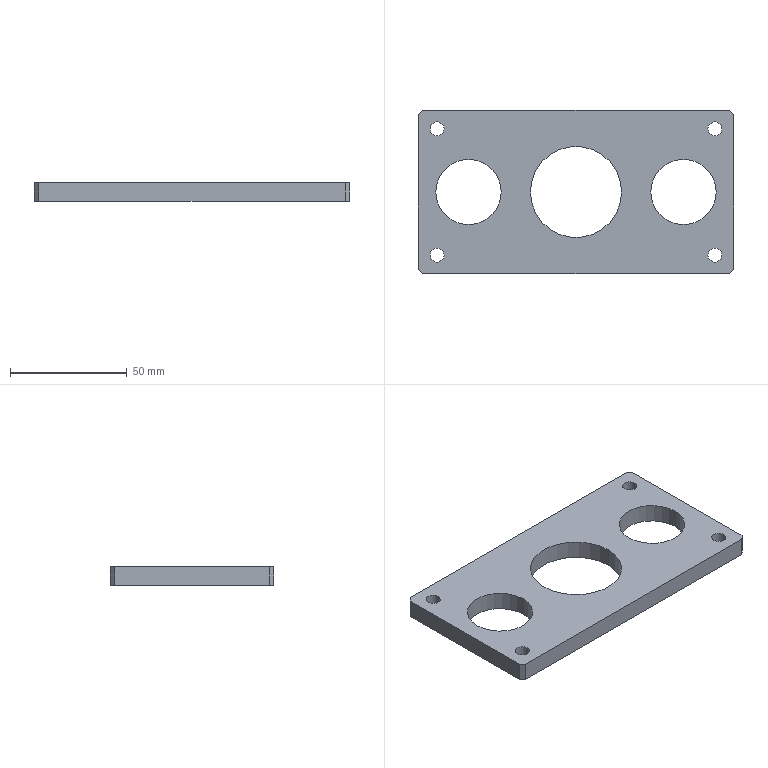Part | SolidWorks | features ICE 3, Chamfer 1, Extrusion 1 | 1 solid | 24 faces | box 135 x 70 x 8 mm | volume 55222 mm3 | cylinder 14 | plane 10 | commonest cylinder face diameters 6 x8 28 x4 39 x2
STEP:
#1=CARTESIAN_POINT('',(56.5,27.,0.));
#2=VERTEX_POINT('',#1);
#3=CARTESIAN_POINT('',(62.5,27.,0.));
#4=VERTEX_POINT('',#3);
#5=CARTESIAN_POINT('',(59.5,27.,0.));
#6=DIRECTION('',(0.,0.,1.));
#7=DIRECTION('',(-1.,0.,0.));
#8=AXIS2_PLACEMENT_3D('',#5,#6,#7);
#9=CIRCLE('',#8,3.);
#10=EDGE_CURVE('',#2,#4,#9,.T.);
#11=ORIENTED_EDGE('',*,*,#10,.F.);
#12=CARTESIAN_POINT('',(56.5,27.,8.));
#13=VERTEX_POINT('',#12);
#14=CARTESIAN_POINT('',(56.5,27.,-0.001));
#15=DIRECTION('',(0.,0.,1.));
#16=VECTOR('',#15,1000.);
#17=LINE('',#14,#16);
#18=EDGE_CURVE('',#2,#13,#17,.T.);
#19=ORIENTED_EDGE('',*,*,#18,.T.);
#20=CARTESIAN_POINT('',(62.5,27.,8.));
#21=VERTEX_POINT('',#20);
#22=CARTESIAN_POINT('',(59.5,27.,8.));
#23=DIRECTION('',(0.,0.,1.));
#24=DIRECTION('',(-1.,0.,0.));
#25=AXIS2_PLACEMENT_3D('',#22,#23,#24);
#26=CIRCLE('',#25,3.);
#27=EDGE_CURVE('',#13,#21,#26,.T.);
#28=ORIENTED_EDGE('',*,*,#27,.T.);
#29=CARTESIAN_POINT('',(62.5,27.,-0.001));
#30=DIRECTION('',(0.,0.,1.));
#31=VECTOR('',#30,1000.);
#32=LINE('',#29,#31);
#33=EDGE_CURVE('',#4,#21,#32,.T.);
#34=ORIENTED_EDGE('',*,*,#33,.F.);
#35=EDGE_LOOP('',(#11,#19,#28,#34));
#36=FACE_OUTER_BOUND('',#35,.T.);
#37=CARTESIAN_POINT('',(59.5,27.,-0.001));
#38=DIRECTION('',(0.,0.,1.));
#39=DIRECTION('',(1.,0.,0.));
#40=AXIS2_PLACEMENT_3D('',#37,#38,#39);
#41=CYLINDRICAL_SURFACE('',#40,3.);
#42=ADVANCED_FACE('',(#36),#41,.F.);
#43=CARTESIAN_POINT('',(56.5,-27.,0.));
#44=VERTEX_POINT('',#43);
#45=CARTESIAN_POINT('',(62.5,-27.,0.));
#46=VERTEX_POINT('',#45);
#47=CARTESIAN_POINT('',(59.5,-27.,0.));
#48=DIRECTION('',(0.,0.,1.));
#49=DIRECTION('',(-1.,0.,0.));
#50=AXIS2_PLACEMENT_3D('',#47,#48,#49);
#51=CIRCLE('',#50,3.);
#52=EDGE_CURVE('',#44,#46,#51,.T.);
#53=ORIENTED_EDGE('',*,*,#52,.F.);
#54=CARTESIAN_POINT('',(56.5,-27.,8.));
#55=VERTEX_POINT('',#54);
#56=CARTESIAN_POINT('',(56.5,-27.,-0.001));
#57=DIRECTION('',(0.,0.,1.));
#58=VECTOR('',#57,1000.);
#59=LINE('',#56,#58);
#60=EDGE_CURVE('',#44,#55,#59,.T.);
#61=ORIENTED_EDGE('',*,*,#60,.T.);
#62=CARTESIAN_POINT('',(62.5,-27.,8.));
#63=VERTEX_POINT('',#62);
#64=CARTESIAN_POINT('',(59.5,-27.,8.));
#65=DIRECTION('',(0.,0.,1.));
#66=DIRECTION('',(-1.,0.,0.));
#67=AXIS2_PLACEMENT_3D('',#64,#65,#66);
#68=CIRCLE('',#67,3.);
#69=EDGE_CURVE('',#55,#63,#68,.T.);
#70=ORIENTED_EDGE('',*,*,#69,.T.);
#71=CARTESIAN_POINT('',(62.5,-27.,-0.001));
#72=DIRECTION('',(0.,0.,1.));
#73=VECTOR('',#72,1000.);
#74=LINE('',#71,#73);
#75=EDGE_CURVE('',#46,#63,#74,.T.);
#76=ORIENTED_EDGE('',*,*,#75,.F.);
#77=EDGE_LOOP('',(#53,#61,#70,#76));
#78=FACE_OUTER_BOUND('',#77,.T.);
#79=CARTESIAN_POINT('',(59.5,-27.,-0.001));
#80=DIRECTION('',(0.,0.,1.));
#81=DIRECTION('',(1.,0.,0.));
#82=AXIS2_PLACEMENT_3D('',#79,#80,#81);
#83=CYLINDRICAL_SURFACE('',#82,3.);
#84=ADVANCED_FACE('',(#78),#83,.F.);
#85=CARTESIAN_POINT('',(-62.5,-27.,0.));
#86=VERTEX_POINT('',#85);
#87=CARTESIAN_POINT('',(-56.5,-27.,0.));
#88=VERTEX_POINT('',#87);
#89=CARTESIAN_POINT('',(-59.5,-27.,0.));
#90=DIRECTION('',(0.,0.,1.));
#91=DIRECTION('',(-1.,0.,0.));
#92=AXIS2_PLACEMENT_3D('',#89,#90,#91);
#93=CIRCLE('',#92,3.);
#94=EDGE_CURVE('',#86,#88,#93,.T.);
#95=ORIENTED_EDGE('',*,*,#94,.F.);
#96=CARTESIAN_POINT('',(-62.5,-27.,8.));
#97=VERTEX_POINT('',#96);
#98=CARTESIAN_POINT('',(-62.5,-27.,-0.001));
#99=DIRECTION('',(0.,0.,1.));
#100=VECTOR('',#99,1000.);
#101=LINE('',#98,#100);
#102=EDGE_CURVE('',#86,#97,#101,.T.);
#103=ORIENTED_EDGE('',*,*,#102,.T.);
#104=CARTESIAN_POINT('',(-56.5,-27.,8.));
#105=VERTEX_POINT('',#104);
#106=CARTESIAN_POINT('',(-59.5,-27.,8.));
#107=DIRECTION('',(0.,0.,1.));
#108=DIRECTION('',(1.,0.,0.));
#109=AXIS2_PLACEMENT_3D('',#106,#107,#108);
#110=CIRCLE('',#109,3.);
#111=EDGE_CURVE('',#97,#105,#110,.T.);
#112=ORIENTED_EDGE('',*,*,#111,.T.);
#113=CARTESIAN_POINT('',(-56.5,-27.,-0.001));
#114=DIRECTION('',(0.,0.,1.));
#115=VECTOR('',#114,1000.);
#116=LINE('',#113,#115);
#117=EDGE_CURVE('',#88,#105,#116,.T.);
#118=ORIENTED_EDGE('',*,*,#117,.F.);
#119=EDGE_LOOP('',(#95,#103,#112,#118));
#120=FACE_OUTER_BOUND('',#119,.T.);
#121=CARTESIAN_POINT('',(-59.5,-27.,-0.001));
#122=DIRECTION('',(0.,0.,1.));
#123=DIRECTION('',(1.,0.,0.));
#124=AXIS2_PLACEMENT_3D('',#121,#122,#123);
#125=CYLINDRICAL_SURFACE('',#124,3.);
#126=ADVANCED_FACE('',(#120),#125,.F.);
#127=CARTESIAN_POINT('',(-62.5,27.,0.));
#128=VERTEX_POINT('',#127);
#129=CARTESIAN_POINT('',(-56.5,27.,0.));
#130=VERTEX_POINT('',#129);
#131=CARTESIAN_POINT('',(-59.5,27.,0.));
#132=DIRECTION('',(0.,0.,1.));
#133=DIRECTION('',(-1.,0.,0.));
#134=AXIS2_PLACEMENT_3D('',#131,#132,#133);
#135=CIRCLE('',#134,3.);
#136=EDGE_CURVE('',#128,#130,#135,.T.);
#137=ORIENTED_EDGE('',*,*,#136,.F.);
#138=CARTESIAN_POINT('',(-62.5,27.,8.));
#139=VERTEX_POINT('',#138);
#140=CARTESIAN_POINT('',(-62.5,27.,-0.001));
#141=DIRECTION('',(0.,0.,1.));
#142=VECTOR('',#141,1000.);
#143=LINE('',#140,#142);
#144=EDGE_CURVE('',#128,#139,#143,.T.);
#145=ORIENTED_EDGE('',*,*,#144,.T.);
#146=CARTESIAN_POINT('',(-56.5,27.,8.));
#147=VERTEX_POINT('',#146);
#148=CARTESIAN_POINT('',(-59.5,27.,8.));
#149=DIRECTION('',(0.,0.,1.));
#150=DIRECTION('',(1.,0.,0.));
#151=AXIS2_PLACEMENT_3D('',#148,#149,#150);
#152=CIRCLE('',#151,3.);
#153=EDGE_CURVE('',#139,#147,#152,.T.);
#154=ORIENTED_EDGE('',*,*,#153,.T.);
#155=CARTESIAN_POINT('',(-56.5,27.,-0.001));
#156=DIRECTION('',(0.,0.,1.));
#157=VECTOR('',#156,1000.);
#158=LINE('',#155,#157);
#159=EDGE_CURVE('',#130,#147,#158,.T.);
#160=ORIENTED_EDGE('',*,*,#159,.F.);
#161=EDGE_LOOP('',(#137,#145,#154,#160));
#162=FACE_OUTER_BOUND('',#161,.T.);
#163=CARTESIAN_POINT('',(-59.5,27.,-0.001));
#164=DIRECTION('',(0.,0.,1.));
#165=DIRECTION('',(1.,0.,0.));
#166=AXIS2_PLACEMENT_3D('',#163,#164,#165);
#167=CYLINDRICAL_SURFACE('',#166,3.);
#168=ADVANCED_FACE('',(#162),#167,.F.);
#169=CARTESIAN_POINT('',(32.,0.,0.));
#170=VERTEX_POINT('',#169);
#171=CARTESIAN_POINT('',(60.,0.,0.));
#172=VERTEX_POINT('',#171);
#173=CARTESIAN_POINT('',(46.,0.,0.));
#174=DIRECTION('',(0.,0.,1.));
#175=DIRECTION('',(-1.,0.,0.));
#176=AXIS2_PLACEMENT_3D('',#173,#174,#175);
#177=CIRCLE('',#176,14.);
#178=EDGE_CURVE('',#170,#172,#177,.T.);
#179=ORIENTED_EDGE('',*,*,#178,.F.);
#180=CARTESIAN_POINT('',(32.,0.,8.));
#181=VERTEX_POINT('',#180);
#182=CARTESIAN_POINT('',(32.,0.,-0.001));
#183=DIRECTION('',(0.,0.,1.));
#184=VECTOR('',#183,1000.);
#185=LINE('',#182,#184);
#186=EDGE_CURVE('',#170,#181,#185,.T.);
#187=ORIENTED_EDGE('',*,*,#186,.T.);
#188=CARTESIAN_POINT('',(60.,0.,8.));
#189=VERTEX_POINT('',#188);
#190=CARTESIAN_POINT('',(46.,0.,8.));
#191=DIRECTION('',(0.,0.,1.));
#192=DIRECTION('',(1.,0.,0.));
#193=AXIS2_PLACEMENT_3D('',#190,#191,#192);
#194=CIRCLE('',#193,14.);
#195=EDGE_CURVE('',#181,#189,#194,.T.);
#196=ORIENTED_EDGE('',*,*,#195,.T.);
#197=CARTESIAN_POINT('',(60.,0.,-0.001));
#198=DIRECTION('',(0.,0.,1.));
#199=VECTOR('',#198,1000.);
#200=LINE('',#197,#199);
#201=EDGE_CURVE('',#172,#189,#200,.T.);
#202=ORIENTED_EDGE('',*,*,#201,.F.);
#203=EDGE_LOOP('',(#179,#187,#196,#202));
#204=FACE_OUTER_BOUND('',#203,.T.);
#205=CARTESIAN_POINT('',(46.,0.,-0.001));
#206=DIRECTION('',(0.,0.,1.));
#207=DIRECTION('',(1.,0.,0.));
#208=AXIS2_PLACEMENT_3D('',#205,#206,#207);
#209=CYLINDRICAL_SURFACE('',#208,14.);
#210=ADVANCED_FACE('',(#204),#209,.F.);
#211=CARTESIAN_POINT('',(-60.,0.,0.));
#212=VERTEX_POINT('',#211);
#213=CARTESIAN_POINT('',(-32.,0.,0.));
#214=VERTEX_POINT('',#213);
#215=CARTESIAN_POINT('',(-46.,0.,0.));
#216=DIRECTION('',(0.,0.,1.));
#217=DIRECTION('',(-1.,0.,0.));
#218=AXIS2_PLACEMENT_3D('',#215,#216,#217);
#219=CIRCLE('',#218,14.);
#220=EDGE_CURVE('',#212,#214,#219,.T.);
#221=ORIENTED_EDGE('',*,*,#220,.F.);
#222=CARTESIAN_POINT('',(-60.,0.,8.));
#223=VERTEX_POINT('',#222);
#224=CARTESIAN_POINT('',(-60.,0.,-0.001));
#225=DIRECTION('',(0.,0.,1.));
#226=VECTOR('',#225,1000.);
#227=LINE('',#224,#226);
#228=EDGE_CURVE('',#212,#223,#227,.T.);
#229=ORIENTED_EDGE('',*,*,#228,.T.);
#230=CARTESIAN_POINT('',(-32.,0.,8.));
#231=VERTEX_POINT('',#230);
#232=CARTESIAN_POINT('',(-46.,0.,8.));
#233=DIRECTION('',(0.,0.,1.));
#234=DIRECTION('',(1.,0.,0.));
#235=AXIS2_PLACEMENT_3D('',#232,#233,#234);
#236=CIRCLE('',#235,14.);
#237=EDGE_CURVE('',#223,#231,#236,.T.);
#238=ORIENTED_EDGE('',*,*,#237,.T.);
#239=CARTESIAN_POINT('',(-32.,0.,-0.001));
#240=DIRECTION('',(0.,0.,1.));
#241=VECTOR('',#240,1000.);
#242=LINE('',#239,#241);
#243=EDGE_CURVE('',#214,#231,#242,.T.);
#244=ORIENTED_EDGE('',*,*,#243,.F.);
#245=EDGE_LOOP('',(#221,#229,#238,#244));
#246=FACE_OUTER_BOUND('',#245,.T.);
#247=CARTESIAN_POINT('',(-46.,0.,-0.001));
#248=DIRECTION('',(0.,0.,1.));
#249=DIRECTION('',(1.,0.,0.));
#250=AXIS2_PLACEMENT_3D('',#247,#248,#249);
#251=CYLINDRICAL_SURFACE('',#250,14.);
#252=ADVANCED_FACE('',(#246),#251,.F.);
#253=CARTESIAN_POINT('',(-19.5,0.,0.));
#254=VERTEX_POINT('',#253);
#255=CARTESIAN_POINT('',(19.5,0.,0.));
#256=VERTEX_POINT('',#255);
#257=CARTESIAN_POINT('',(0.,0.,0.));
#258=DIRECTION('',(0.,0.,1.));
#259=DIRECTION('',(-1.,0.,0.));
#260=AXIS2_PLACEMENT_3D('',#257,#258,#259);
#261=CIRCLE('',#260,19.5);
#262=EDGE_CURVE('',#254,#256,#261,.T.);
#263=ORIENTED_EDGE('',*,*,#262,.F.);
#264=CARTESIAN_POINT('',(-19.5,0.,8.));
#265=VERTEX_POINT('',#264);
#266=CARTESIAN_POINT('',(-19.5,0.,-0.001));
#267=DIRECTION('',(0.,0.,1.));
#268=VECTOR('',#267,1000.);
#269=LINE('',#266,#268);
#270=EDGE_CURVE('',#254,#265,#269,.T.);
#271=ORIENTED_EDGE('',*,*,#270,.T.);
#272=CARTESIAN_POINT('',(19.5,0.,8.));
#273=VERTEX_POINT('',#272);
#274=CARTESIAN_POINT('',(0.,0.,8.));
#275=DIRECTION('',(0.,0.,1.));
#276=DIRECTION('',(1.,0.,0.));
#277=AXIS2_PLACEMENT_3D('',#274,#275,#276);
#278=CIRCLE('',#277,19.5);
#279=EDGE_CURVE('',#265,#273,#278,.T.);
#280=ORIENTED_EDGE('',*,*,#279,.T.);
#281=CARTESIAN_POINT('',(19.5,0.,-0.001));
#282=DIRECTION('',(0.,0.,1.));
#283=VECTOR('',#282,1000.);
#284=LINE('',#281,#283);
#285=EDGE_CURVE('',#256,#273,#284,.T.);
#286=ORIENTED_EDGE('',*,*,#285,.F.);
#287=EDGE_LOOP('',(#263,#271,#280,#286));
#288=FACE_OUTER_BOUND('',#287,.T.);
#289=CARTESIAN_POINT('',(0.,0.,-0.001));
#290=DIRECTION('',(0.,0.,1.));
#291=DIRECTION('',(1.,0.,0.));
#292=AXIS2_PLACEMENT_3D('',#289,#290,#291);
#293=CYLINDRICAL_SURFACE('',#292,19.5);
#294=ADVANCED_FACE('',(#288),#293,.F.);
#295=CARTESIAN_POINT('',(67.5,-33.,8.));
#296=VERTEX_POINT('',#295);
#297=CARTESIAN_POINT('',(67.5,33.,8.));
#298=VERTEX_POINT('',#297);
#299=CARTESIAN_POINT('',(67.5,-35.,8.));
#300=DIRECTION('',(0.,1.,0.));
#301=VECTOR('',#300,1000.);
#302=LINE('',#299,#301);
#303=EDGE_CURVE('',#296,#298,#302,.T.);
#304=ORIENTED_EDGE('',*,*,#303,.F.);
#305=CARTESIAN_POINT('',(67.5,-33.,0.));
#306=VERTEX_POINT('',#305);
#307=CARTESIAN_POINT('',(67.5,-33.,8.));
#308=DIRECTION('',(0.,0.,-1.));
#309=VECTOR('',#308,1000.);
#310=LINE('',#307,#309);
#311=EDGE_CURVE('',#296,#306,#310,.T.);
#312=ORIENTED_EDGE('',*,*,#311,.T.);
#313=CARTESIAN_POINT('',(67.5,33.,0.));
#314=VERTEX_POINT('',#313);
#315=CARTESIAN_POINT('',(67.5,-35.,0.));
#316=DIRECTION('',(0.,1.,0.));
#317=VECTOR('',#316,1000.);
#318=LINE('',#315,#317);
#319=EDGE_CURVE('',#306,#314,#318,.T.);
#320=ORIENTED_EDGE('',*,*,#319,.T.);
#321=CARTESIAN_POINT('',(67.5,33.,8.));
#322=DIRECTION('',(0.,0.,1.));
#323=VECTOR('',#322,1000.);
#324=LINE('',#321,#323);
#325=EDGE_CURVE('',#314,#298,#324,.T.);
#326=ORIENTED_EDGE('',*,*,#325,.T.);
#327=EDGE_LOOP('',(#304,#312,#320,#326));
#328=FACE_OUTER_BOUND('',#327,.T.);
#329=CARTESIAN_POINT('',(67.5,-35.,8.));
#330=DIRECTION('',(-1.,0.,0.));
#331=DIRECTION('',(0.,0.,1.));
#332=AXIS2_PLACEMENT_3D('',#329,#330,#331);
#333=PLANE('',#332);
#334=ADVANCED_FACE('',(#328),#333,.F.);
#335=CARTESIAN_POINT('',(65.5,35.,8.));
#336=VERTEX_POINT('',#335);
#337=CARTESIAN_POINT('',(-65.5,35.,8.));
#338=VERTEX_POINT('',#337);
#339=CARTESIAN_POINT('',(-67.5,35.,8.));
#340=DIRECTION('',(-1.,0.,0.));
#341=VECTOR('',#340,1000.);
#342=LINE('',#339,#341);
#343=EDGE_CURVE('',#336,#338,#342,.T.);
#344=ORIENTED_EDGE('',*,*,#343,.F.);
#345=CARTESIAN_POINT('',(65.5,35.,0.));
#346=VERTEX_POINT('',#345);
#347=CARTESIAN_POINT('',(65.5,35.,8.));
#348=DIRECTION('',(0.,0.,-1.));
#349=VECTOR('',#348,1000.);
#350=LINE('',#347,#349);
#351=EDGE_CURVE('',#336,#346,#350,.T.);
#352=ORIENTED_EDGE('',*,*,#351,.T.);
#353=CARTESIAN_POINT('',(-65.5,35.,0.));
#354=VERTEX_POINT('',#353);
#355=CARTESIAN_POINT('',(-67.5,35.,0.));
#356=DIRECTION('',(-1.,0.,0.));
#357=VECTOR('',#356,1000.);
#358=LINE('',#355,#357);
#359=EDGE_CURVE('',#346,#354,#358,.T.);
#360=ORIENTED_EDGE('',*,*,#359,.T.);
#361=CARTESIAN_POINT('',(-65.5,35.,8.));
#362=DIRECTION('',(0.,0.,1.));
#363=VECTOR('',#362,1000.);
#364=LINE('',#361,#363);
#365=EDGE_CURVE('',#354,#338,#364,.T.);
#366=ORIENTED_EDGE('',*,*,#365,.T.);
#367=EDGE_LOOP('',(#344,#352,#360,#366));
#368=FACE_OUTER_BOUND('',#367,.T.);
#369=CARTESIAN_POINT('',(-67.5,35.,8.));
#370=DIRECTION('',(0.,-1.,0.));
#371=DIRECTION('',(0.,0.,-1.));
#372=AXIS2_PLACEMENT_3D('',#369,#370,#371);
#373=PLANE('',#372);
#374=ADVANCED_FACE('',(#368),#373,.F.);
#375=CARTESIAN_POINT('',(-67.5,33.,0.));
#376=VERTEX_POINT('',#375);
#377=CARTESIAN_POINT('',(-67.5,-33.,0.));
#378=VERTEX_POINT('',#377);
#379=CARTESIAN_POINT('',(-67.5,-35.,0.));
#380=DIRECTION('',(0.,-1.,0.));
#381=VECTOR('',#380,1000.);
#382=LINE('',#379,#381);
#383=EDGE_CURVE('',#376,#378,#382,.T.);
#384=ORIENTED_EDGE('',*,*,#383,.T.);
#385=CARTESIAN_POINT('',(-67.5,-33.,8.));
#386=VERTEX_POINT('',#385);
#387=CARTESIAN_POINT('',(-67.5,-33.,8.));
#388=DIRECTION('',(0.,0.,1.));
#389=VECTOR('',#388,1000.);
#390=LINE('',#387,#389);
#391=EDGE_CURVE('',#378,#386,#390,.T.);
#392=ORIENTED_EDGE('',*,*,#391,.T.);
#393=CARTESIAN_POINT('',(-67.5,33.,8.));
#394=VERTEX_POINT('',#393);
#395=CARTESIAN_POINT('',(-67.5,-35.,8.));
#396=DIRECTION('',(0.,-1.,0.));
#397=VECTOR('',#396,1000.);
#398=LINE('',#395,#397);
#399=EDGE_CURVE('',#394,#386,#398,.T.);
#400=ORIENTED_EDGE('',*,*,#399,.F.);
#401=CARTESIAN_POINT('',(-67.5,33.,8.));
#402=DIRECTION('',(0.,0.,-1.));
#403=VECTOR('',#402,1000.);
#404=LINE('',#401,#403);
#405=EDGE_CURVE('',#394,#376,#404,.T.);
#406=ORIENTED_EDGE('',*,*,#405,.T.);
#407=EDGE_LOOP('',(#384,#392,#400,#406));
#408=FACE_OUTER_BOUND('',#407,.T.);
#409=CARTESIAN_POINT('',(-67.5,-35.,8.));
#410=DIRECTION('',(1.,0.,0.));
#411=DIRECTION('',(0.,0.,-1.));
#412=AXIS2_PLACEMENT_3D('',#409,#410,#411);
#413=PLANE('',#412);
#414=ADVANCED_FACE('',(#408),#413,.F.);
#415=CARTESIAN_POINT('',(-65.5,-35.,8.));
#416=VERTEX_POINT('',#415);
#417=CARTESIAN_POINT('',(65.5,-35.,8.));
#418=VERTEX_POINT('',#417);
#419=CARTESIAN_POINT('',(-67.5,-35.,8.));
#420=DIRECTION('',(1.,0.,0.));
#421=VECTOR('',#420,1000.);
#422=LINE('',#419,#421);
#423=EDGE_CURVE('',#416,#418,#422,.T.);
#424=ORIENTED_EDGE('',*,*,#423,.F.);
#425=CARTESIAN_POINT('',(-65.5,-35.,0.));
#426=VERTEX_POINT('',#425);
#427=CARTESIAN_POINT('',(-65.5,-35.,8.));
#428=DIRECTION('',(0.,0.,-1.));
#429=VECTOR('',#428,1000.);
#430=LINE('',#427,#429);
#431=EDGE_CURVE('',#416,#426,#430,.T.);
#432=ORIENTED_EDGE('',*,*,#431,.T.);
#433=CARTESIAN_POINT('',(65.5,-35.,0.));
#434=VERTEX_POINT('',#433);
#435=CARTESIAN_POINT('',(-67.5,-35.,0.));
#436=DIRECTION('',(1.,0.,0.));
#437=VECTOR('',#436,1000.);
#438=LINE('',#435,#437);
#439=EDGE_CURVE('',#426,#434,#438,.T.);
#440=ORIENTED_EDGE('',*,*,#439,.T.);
#441=CARTESIAN_POINT('',(65.5,-35.,8.));
#442=DIRECTION('',(0.,0.,1.));
#443=VECTOR('',#442,1000.);
#444=LINE('',#441,#443);
#445=EDGE_CURVE('',#434,#418,#444,.T.);
#446=ORIENTED_EDGE('',*,*,#445,.T.);
#447=EDGE_LOOP('',(#424,#432,#440,#446));
#448=FACE_OUTER_BOUND('',#447,.T.);
#449=CARTESIAN_POINT('',(-67.5,-35.,8.));
#450=DIRECTION('',(0.,1.,0.));
#451=DIRECTION('',(0.,0.,1.));
#452=AXIS2_PLACEMENT_3D('',#449,#450,#451);
#453=PLANE('',#452);
#454=ADVANCED_FACE('',(#448),#453,.F.);
#455=CARTESIAN_POINT('',(59.5,27.,8.));
#456=DIRECTION('',(0.,0.,1.));
#457=DIRECTION('',(-1.,0.,0.));
#458=AXIS2_PLACEMENT_3D('',#455,#456,#457);
#459=CIRCLE('',#458,3.);
#460=EDGE_CURVE('',#21,#13,#459,.T.);
#461=ORIENTED_EDGE('',*,*,#460,.F.);
#462=ORIENTED_EDGE('',*,*,#27,.F.);
#463=EDGE_LOOP('',(#461,#462));
#464=FACE_BOUND('',#463,.T.);
#465=CARTESIAN_POINT('',(59.5,-27.,8.));
#466=DIRECTION('',(0.,0.,1.));
#467=DIRECTION('',(-1.,0.,0.));
#468=AXIS2_PLACEMENT_3D('',#465,#466,#467);
#469=CIRCLE('',#468,3.);
#470=EDGE_CURVE('',#63,#55,#469,.T.);
#471=ORIENTED_EDGE('',*,*,#470,.F.);
#472=ORIENTED_EDGE('',*,*,#69,.F.);
#473=EDGE_LOOP('',(#471,#472));
#474=FACE_BOUND('',#473,.T.);
#475=CARTESIAN_POINT('',(-59.5,-27.,8.));
#476=DIRECTION('',(0.,0.,1.));
#477=DIRECTION('',(1.,0.,0.));
#478=AXIS2_PLACEMENT_3D('',#475,#476,#477);
#479=CIRCLE('',#478,3.);
#480=EDGE_CURVE('',#105,#97,#479,.T.);
#481=ORIENTED_EDGE('',*,*,#480,.F.);
#482=ORIENTED_EDGE('',*,*,#111,.F.);
#483=EDGE_LOOP('',(#481,#482));
#484=FACE_BOUND('',#483,.T.);
#485=CARTESIAN_POINT('',(-59.5,27.,8.));
#486=DIRECTION('',(0.,0.,1.));
#487=DIRECTION('',(1.,0.,0.));
#488=AXIS2_PLACEMENT_3D('',#485,#486,#487);
#489=CIRCLE('',#488,3.);
#490=EDGE_CURVE('',#147,#139,#489,.T.);
#491=ORIENTED_EDGE('',*,*,#490,.F.);
#492=ORIENTED_EDGE('',*,*,#153,.F.);
#493=EDGE_LOOP('',(#491,#492));
#494=FACE_BOUND('',#493,.T.);
#495=CARTESIAN_POINT('',(46.,0.,8.));
#496=DIRECTION('',(0.,0.,1.));
#497=DIRECTION('',(1.,0.,0.));
#498=AXIS2_PLACEMENT_3D('',#495,#496,#497);
#499=CIRCLE('',#498,14.);
#500=EDGE_CURVE('',#189,#181,#499,.T.);
#501=ORIENTED_EDGE('',*,*,#500,.F.);
#502=ORIENTED_EDGE('',*,*,#195,.F.);
#503=EDGE_LOOP('',(#501,#502));
#504=FACE_BOUND('',#503,.T.);
#505=CARTESIAN_POINT('',(-46.,0.,8.));
#506=DIRECTION('',(0.,0.,1.));
#507=DIRECTION('',(1.,0.,0.));
#508=AXIS2_PLACEMENT_3D('',#505,#506,#507);
#509=CIRCLE('',#508,14.);
#510=EDGE_CURVE('',#231,#223,#509,.T.);
#511=ORIENTED_EDGE('',*,*,#510,.F.);
#512=ORIENTED_EDGE('',*,*,#237,.F.);
#513=EDGE_LOOP('',(#511,#512));
#514=FACE_BOUND('',#513,.T.);
#515=CARTESIAN_POINT('',(0.,0.,8.));
#516=DIRECTION('',(0.,0.,1.));
#517=DIRECTION('',(1.,0.,0.));
#518=AXIS2_PLACEMENT_3D('',#515,#516,#517);
#519=CIRCLE('',#518,19.5);
#520=EDGE_CURVE('',#273,#265,#519,.T.);
#521=ORIENTED_EDGE('',*,*,#520,.F.);
#522=ORIENTED_EDGE('',*,*,#279,.F.);
#523=EDGE_LOOP('',(#521,#522));
#524=FACE_BOUND('',#523,.T.);
#525=ORIENTED_EDGE('',*,*,#399,.T.);
#526=CARTESIAN_POINT('',(-65.5,-35.,8.));
#527=DIRECTION('',(0.7071,-0.7071,0.));
#528=VECTOR('',#527,1000.);
#529=LINE('',#526,#528);
#530=EDGE_CURVE('',#386,#416,#529,.T.);
#531=ORIENTED_EDGE('',*,*,#530,.T.);
#532=ORIENTED_EDGE('',*,*,#423,.T.);
#533=CARTESIAN_POINT('',(67.5,-33.,8.));
#534=DIRECTION('',(0.7071,0.7071,0.));
#535=VECTOR('',#534,1000.);
#536=LINE('',#533,#535);
#537=EDGE_CURVE('',#418,#296,#536,.T.);
#538=ORIENTED_EDGE('',*,*,#537,.T.);
#539=ORIENTED_EDGE('',*,*,#303,.T.);
#540=CARTESIAN_POINT('',(65.5,35.,8.));
#541=DIRECTION('',(-0.7071,0.7071,0.));
#542=VECTOR('',#541,1000.);
#543=LINE('',#540,#542);
#544=EDGE_CURVE('',#298,#336,#543,.T.);
#545=ORIENTED_EDGE('',*,*,#544,.T.);
#546=ORIENTED_EDGE('',*,*,#343,.T.);
#547=CARTESIAN_POINT('',(-67.5,33.,8.));
#548=DIRECTION('',(-0.7071,-0.7071,0.));
#549=VECTOR('',#548,1000.);
#550=LINE('',#547,#549);
#551=EDGE_CURVE('',#338,#394,#550,.T.);
#552=ORIENTED_EDGE('',*,*,#551,.T.);
#553=EDGE_LOOP('',(#525,#531,#532,#538,#539,#545,#546,#552));
#554=FACE_OUTER_BOUND('',#553,.T.);
#555=CARTESIAN_POINT('',(0.,0.,8.));
#556=DIRECTION('',(0.,0.,-1.));
#557=DIRECTION('',(-1.,0.,0.));
#558=AXIS2_PLACEMENT_3D('',#555,#556,#557);
#559=PLANE('',#558);
#560=ADVANCED_FACE('',(#464,#474,#484,#494,#504,#514,#524,#554),#559,.F.);
#561=CARTESIAN_POINT('',(59.5,27.,0.));
#562=DIRECTION('',(0.,0.,1.));
#563=DIRECTION('',(-1.,0.,0.));
#564=AXIS2_PLACEMENT_3D('',#561,#562,#563);
#565=CIRCLE('',#564,3.);
#566=EDGE_CURVE('',#4,#2,#565,.T.);
#567=ORIENTED_EDGE('',*,*,#566,.T.);
#568=ORIENTED_EDGE('',*,*,#10,.T.);
#569=EDGE_LOOP('',(#567,#568));
#570=FACE_BOUND('',#569,.T.);
#571=CARTESIAN_POINT('',(59.5,-27.,0.));
#572=DIRECTION('',(0.,0.,1.));
#573=DIRECTION('',(-1.,0.,0.));
#574=AXIS2_PLACEMENT_3D('',#571,#572,#573);
#575=CIRCLE('',#574,3.);
#576=EDGE_CURVE('',#46,#44,#575,.T.);
#577=ORIENTED_EDGE('',*,*,#576,.T.);
#578=ORIENTED_EDGE('',*,*,#52,.T.);
#579=EDGE_LOOP('',(#577,#578));
#580=FACE_BOUND('',#579,.T.);
#581=CARTESIAN_POINT('',(-59.5,-27.,0.));
#582=DIRECTION('',(0.,0.,1.));
#583=DIRECTION('',(-1.,0.,0.));
#584=AXIS2_PLACEMENT_3D('',#581,#582,#583);
#585=CIRCLE('',#584,3.);
#586=EDGE_CURVE('',#88,#86,#585,.T.);
#587=ORIENTED_EDGE('',*,*,#586,.T.);
#588=ORIENTED_EDGE('',*,*,#94,.T.);
#589=EDGE_LOOP('',(#587,#588));
#590=FACE_BOUND('',#589,.T.);
#591=CARTESIAN_POINT('',(-59.5,27.,0.));
#592=DIRECTION('',(0.,0.,1.));
#593=DIRECTION('',(-1.,0.,0.));
#594=AXIS2_PLACEMENT_3D('',#591,#592,#593);
#595=CIRCLE('',#594,3.);
#596=EDGE_CURVE('',#130,#128,#595,.T.);
#597=ORIENTED_EDGE('',*,*,#596,.T.);
#598=ORIENTED_EDGE('',*,*,#136,.T.);
#599=EDGE_LOOP('',(#597,#598));
#600=FACE_BOUND('',#599,.T.);
#601=CARTESIAN_POINT('',(46.,0.,0.));
#602=DIRECTION('',(0.,0.,1.));
#603=DIRECTION('',(-1.,0.,0.));
#604=AXIS2_PLACEMENT_3D('',#601,#602,#603);
#605=CIRCLE('',#604,14.);
#606=EDGE_CURVE('',#172,#170,#605,.T.);
#607=ORIENTED_EDGE('',*,*,#606,.T.);
#608=ORIENTED_EDGE('',*,*,#178,.T.);
#609=EDGE_LOOP('',(#607,#608));
#610=FACE_BOUND('',#609,.T.);
#611=CARTESIAN_POINT('',(-46.,0.,0.));
#612=DIRECTION('',(0.,0.,1.));
#613=DIRECTION('',(-1.,0.,0.));
#614=AXIS2_PLACEMENT_3D('',#611,#612,#613);
#615=CIRCLE('',#614,14.);
#616=EDGE_CURVE('',#214,#212,#615,.T.);
#617=ORIENTED_EDGE('',*,*,#616,.T.);
#618=ORIENTED_EDGE('',*,*,#220,.T.);
#619=EDGE_LOOP('',(#617,#618));
#620=FACE_BOUND('',#619,.T.);
#621=CARTESIAN_POINT('',(0.,0.,0.));
#622=DIRECTION('',(0.,0.,1.));
#623=DIRECTION('',(-1.,0.,0.));
#624=AXIS2_PLACEMENT_3D('',#621,#622,#623);
#625=CIRCLE('',#624,19.5);
#626=EDGE_CURVE('',#256,#254,#625,.T.);
#627=ORIENTED_EDGE('',*,*,#626,.T.);
#628=ORIENTED_EDGE('',*,*,#262,.T.);
#629=EDGE_LOOP('',(#627,#628));
#630=FACE_BOUND('',#629,.T.);
#631=ORIENTED_EDGE('',*,*,#439,.F.);
#632=CARTESIAN_POINT('',(-50.25,-50.25,0.));
#633=DIRECTION('',(-0.7071,0.7071,0.));
#634=VECTOR('',#633,1000.);
#635=LINE('',#632,#634);
#636=EDGE_CURVE('',#426,#378,#635,.T.);
#637=ORIENTED_EDGE('',*,*,#636,.T.);
#638=ORIENTED_EDGE('',*,*,#383,.F.);
#639=CARTESIAN_POINT('',(-50.25,50.25,0.));
#640=DIRECTION('',(0.7071,0.7071,0.));
#641=VECTOR('',#640,1000.);
#642=LINE('',#639,#641);
#643=EDGE_CURVE('',#376,#354,#642,.T.);
#644=ORIENTED_EDGE('',*,*,#643,.T.);
#645=ORIENTED_EDGE('',*,*,#359,.F.);
#646=CARTESIAN_POINT('',(50.25,50.25,0.));
#647=DIRECTION('',(0.7071,-0.7071,0.));
#648=VECTOR('',#647,1000.);
#649=LINE('',#646,#648);
#650=EDGE_CURVE('',#346,#314,#649,.T.);
#651=ORIENTED_EDGE('',*,*,#650,.T.);
#652=ORIENTED_EDGE('',*,*,#319,.F.);
#653=CARTESIAN_POINT('',(50.25,-50.25,0.));
#654=DIRECTION('',(-0.7071,-0.7071,0.));
#655=VECTOR('',#654,1000.);
#656=LINE('',#653,#655);
#657=EDGE_CURVE('',#306,#434,#656,.T.);
#658=ORIENTED_EDGE('',*,*,#657,.T.);
#659=EDGE_LOOP('',(#631,#637,#638,#644,#645,#651,#652,#658));
#660=FACE_OUTER_BOUND('',#659,.T.);
#661=CARTESIAN_POINT('',(0.,0.,0.));
#662=DIRECTION('',(0.,0.,-1.));
#663=DIRECTION('',(-1.,0.,0.));
#664=AXIS2_PLACEMENT_3D('',#661,#662,#663);
#665=PLANE('',#664);
#666=ADVANCED_FACE('',(#570,#580,#590,#600,#610,#620,#630,#660),#665,.T.);
#667=ORIENTED_EDGE('',*,*,#270,.F.);
#668=ORIENTED_EDGE('',*,*,#626,.F.);
#669=ORIENTED_EDGE('',*,*,#285,.T.);
#670=ORIENTED_EDGE('',*,*,#520,.T.);
#671=EDGE_LOOP('',(#667,#668,#669,#670));
#672=FACE_OUTER_BOUND('',#671,.T.);
#673=CARTESIAN_POINT('',(0.,0.,-0.001));
#674=DIRECTION('',(0.,0.,1.));
#675=DIRECTION('',(1.,0.,0.));
#676=AXIS2_PLACEMENT_3D('',#673,#674,#675);
#677=CYLINDRICAL_SURFACE('',#676,19.5);
#678=ADVANCED_FACE('',(#672),#677,.F.);
#679=ORIENTED_EDGE('',*,*,#228,.F.);
#680=ORIENTED_EDGE('',*,*,#616,.F.);
#681=ORIENTED_EDGE('',*,*,#243,.T.);
#682=ORIENTED_EDGE('',*,*,#510,.T.);
#683=EDGE_LOOP('',(#679,#680,#681,#682));
#684=FACE_OUTER_BOUND('',#683,.T.);
#685=CARTESIAN_POINT('',(-46.,0.,-0.001));
#686=DIRECTION('',(0.,0.,1.));
#687=DIRECTION('',(1.,0.,0.));
#688=AXIS2_PLACEMENT_3D('',#685,#686,#687);
#689=CYLINDRICAL_SURFACE('',#688,14.);
#690=ADVANCED_FACE('',(#684),#689,.F.);
#691=ORIENTED_EDGE('',*,*,#186,.F.);
#692=ORIENTED_EDGE('',*,*,#606,.F.);
#693=ORIENTED_EDGE('',*,*,#201,.T.);
#694=ORIENTED_EDGE('',*,*,#500,.T.);
#695=EDGE_LOOP('',(#691,#692,#693,#694));
#696=FACE_OUTER_BOUND('',#695,.T.);
#697=CARTESIAN_POINT('',(46.,0.,-0.001));
#698=DIRECTION('',(0.,0.,1.));
#699=DIRECTION('',(1.,0.,0.));
#700=AXIS2_PLACEMENT_3D('',#697,#698,#699);
#701=CYLINDRICAL_SURFACE('',#700,14.);
#702=ADVANCED_FACE('',(#696),#701,.F.);
#703=ORIENTED_EDGE('',*,*,#144,.F.);
#704=ORIENTED_EDGE('',*,*,#596,.F.);
#705=ORIENTED_EDGE('',*,*,#159,.T.);
#706=ORIENTED_EDGE('',*,*,#490,.T.);
#707=EDGE_LOOP('',(#703,#704,#705,#706));
#708=FACE_OUTER_BOUND('',#707,.T.);
#709=CARTESIAN_POINT('',(-59.5,27.,-0.001));
#710=DIRECTION('',(0.,0.,1.));
#711=DIRECTION('',(1.,0.,0.));
#712=AXIS2_PLACEMENT_3D('',#709,#710,#711);
#713=CYLINDRICAL_SURFACE('',#712,3.);
#714=ADVANCED_FACE('',(#708),#713,.F.);
#715=ORIENTED_EDGE('',*,*,#102,.F.);
#716=ORIENTED_EDGE('',*,*,#586,.F.);
#717=ORIENTED_EDGE('',*,*,#117,.T.);
#718=ORIENTED_EDGE('',*,*,#480,.T.);
#719=EDGE_LOOP('',(#715,#716,#717,#718));
#720=FACE_OUTER_BOUND('',#719,.T.);
#721=CARTESIAN_POINT('',(-59.5,-27.,-0.001));
#722=DIRECTION('',(0.,0.,1.));
#723=DIRECTION('',(1.,0.,0.));
#724=AXIS2_PLACEMENT_3D('',#721,#722,#723);
#725=CYLINDRICAL_SURFACE('',#724,3.);
#726=ADVANCED_FACE('',(#720),#725,.F.);
#727=ORIENTED_EDGE('',*,*,#60,.F.);
#728=ORIENTED_EDGE('',*,*,#576,.F.);
#729=ORIENTED_EDGE('',*,*,#75,.T.);
#730=ORIENTED_EDGE('',*,*,#470,.T.);
#731=EDGE_LOOP('',(#727,#728,#729,#730));
#732=FACE_OUTER_BOUND('',#731,.T.);
#733=CARTESIAN_POINT('',(59.5,-27.,-0.001));
#734=DIRECTION('',(0.,0.,1.));
#735=DIRECTION('',(1.,0.,0.));
#736=AXIS2_PLACEMENT_3D('',#733,#734,#735);
#737=CYLINDRICAL_SURFACE('',#736,3.);
#738=ADVANCED_FACE('',(#732),#737,.F.);
#739=ORIENTED_EDGE('',*,*,#18,.F.);
#740=ORIENTED_EDGE('',*,*,#566,.F.);
#741=ORIENTED_EDGE('',*,*,#33,.T.);
#742=ORIENTED_EDGE('',*,*,#460,.T.);
#743=EDGE_LOOP('',(#739,#740,#741,#742));
#744=FACE_OUTER_BOUND('',#743,.T.);
#745=CARTESIAN_POINT('',(59.5,27.,-0.001));
#746=DIRECTION('',(0.,0.,1.));
#747=DIRECTION('',(1.,0.,0.));
#748=AXIS2_PLACEMENT_3D('',#745,#746,#747);
#749=CYLINDRICAL_SURFACE('',#748,3.);
#750=ADVANCED_FACE('',(#744),#749,.F.);
#751=ORIENTED_EDGE('',*,*,#530,.F.);
#752=ORIENTED_EDGE('',*,*,#391,.F.);
#753=ORIENTED_EDGE('',*,*,#636,.F.);
#754=ORIENTED_EDGE('',*,*,#431,.F.);
#755=EDGE_LOOP('',(#751,#752,#753,#754));
#756=FACE_OUTER_BOUND('',#755,.T.);
#757=CARTESIAN_POINT('',(-65.5,-35.,8.));
#758=DIRECTION('',(0.7071,0.7071,0.));
#759=DIRECTION('',(0.,0.,-1.));
#760=AXIS2_PLACEMENT_3D('',#757,#758,#759);
#761=PLANE('',#760);
#762=ADVANCED_FACE('',(#756),#761,.F.);
#763=ORIENTED_EDGE('',*,*,#537,.F.);
#764=ORIENTED_EDGE('',*,*,#445,.F.);
#765=ORIENTED_EDGE('',*,*,#657,.F.);
#766=ORIENTED_EDGE('',*,*,#311,.F.);
#767=EDGE_LOOP('',(#763,#764,#765,#766));
#768=FACE_OUTER_BOUND('',#767,.T.);
#769=CARTESIAN_POINT('',(67.5,-33.,8.));
#770=DIRECTION('',(-0.7071,0.7071,0.));
#771=DIRECTION('',(0.,0.,-1.));
#772=AXIS2_PLACEMENT_3D('',#769,#770,#771);
#773=PLANE('',#772);
#774=ADVANCED_FACE('',(#768),#773,.F.);
#775=ORIENTED_EDGE('',*,*,#544,.F.);
#776=ORIENTED_EDGE('',*,*,#325,.F.);
#777=ORIENTED_EDGE('',*,*,#650,.F.);
#778=ORIENTED_EDGE('',*,*,#351,.F.);
#779=EDGE_LOOP('',(#775,#776,#777,#778));
#780=FACE_OUTER_BOUND('',#779,.T.);
#781=CARTESIAN_POINT('',(65.5,35.,8.));
#782=DIRECTION('',(-0.7071,-0.7071,0.));
#783=DIRECTION('',(0.,0.,-1.));
#784=AXIS2_PLACEMENT_3D('',#781,#782,#783);
#785=PLANE('',#784);
#786=ADVANCED_FACE('',(#780),#785,.F.);
#787=ORIENTED_EDGE('',*,*,#551,.F.);
#788=ORIENTED_EDGE('',*,*,#365,.F.);
#789=ORIENTED_EDGE('',*,*,#643,.F.);
#790=ORIENTED_EDGE('',*,*,#405,.F.);
#791=EDGE_LOOP('',(#787,#788,#789,#790));
#792=FACE_OUTER_BOUND('',#791,.T.);
#793=CARTESIAN_POINT('',(-67.5,33.,8.));
#794=DIRECTION('',(0.7071,-0.7071,0.));
#795=DIRECTION('',(0.,0.,-1.));
#796=AXIS2_PLACEMENT_3D('',#793,#794,#795);
#797=PLANE('',#796);
#798=ADVANCED_FACE('',(#792),#797,.F.);
#799=CLOSED_SHELL('',(#42,#84,#126,#168,#210,#252,#294,#334,#374,#414,#454,#560,#666,#678,#690,#702,#714,#726,#738,#750,#762,#774,#786,#798));
#800=MANIFOLD_SOLID_BREP('',#799);
#801=CARTESIAN_POINT('',(0.,0.,0.));
#802=DIRECTION('',(0.,0.,1.));
#803=DIRECTION('',(1.,0.,0.));
#804=AXIS2_PLACEMENT_3D('',#801,#802,#803);
#805=(LENGTH_UNIT()NAMED_UNIT(*)SI_UNIT(.MILLI.,.METRE.));
#806=UNCERTAINTY_MEASURE_WITH_UNIT(LENGTH_MEASURE(0.00001),#805,'','');
#807=(NAMED_UNIT(*)PLANE_ANGLE_UNIT()SI_UNIT($,.RADIAN.));
#808=(NAMED_UNIT(*)SI_UNIT($,.STERADIAN.)SOLID_ANGLE_UNIT());
#809=(GEOMETRIC_REPRESENTATION_CONTEXT(3)GLOBAL_UNCERTAINTY_ASSIGNED_CONTEXT((#806))GLOBAL_UNIT_ASSIGNED_CONTEXT((#805,#807,#808))REPRESENTATION_CONTEXT('',''));
#810=ADVANCED_BREP_SHAPE_REPRESENTATION('',(#800,#804),#809);